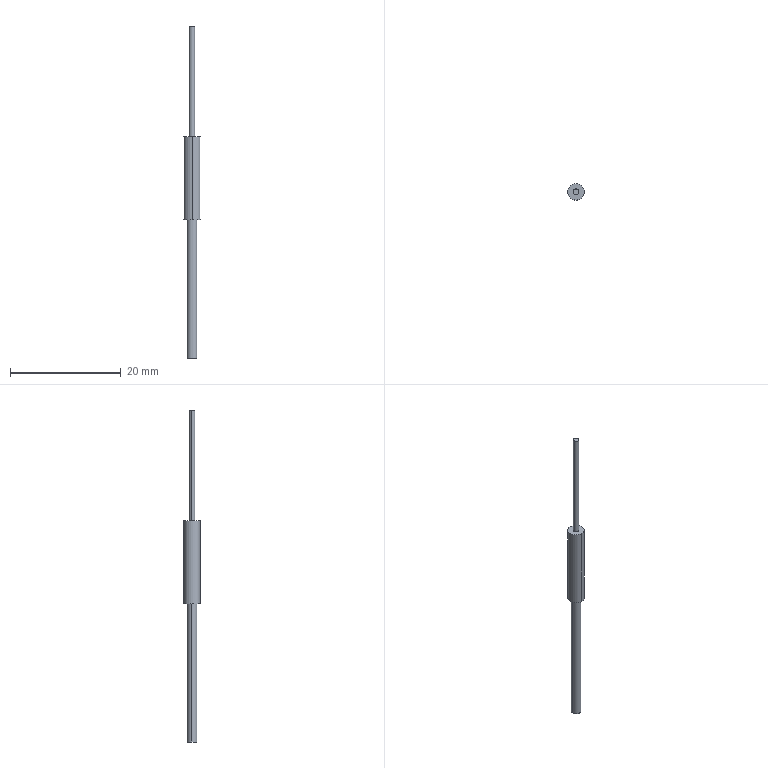Part | SolidWorks | features BaseBody 1 | 1 solid | 10 faces | box 3 x 3 x 60 mm | volume 185.354 mm3 | cylinder 6 | plane 4 | commonest cylinder face diameters 1 x2 1.8 x2 3 x2
STEP:
#1=CARTESIAN_POINT('',(0.03543,0.,-0.9843));
#2=VERTEX_POINT('',#1);
#3=CARTESIAN_POINT('',(-0.03543,0.,-0.9843));
#4=VERTEX_POINT('',#3);
#5=CARTESIAN_POINT('',(0.,0.,-0.9843));
#6=DIRECTION('',(0.,0.,1.));
#7=DIRECTION('',(1.,0.,0.));
#8=AXIS2_PLACEMENT_3D('',#5,#6,#7);
#9=CIRCLE('',#8,0.03543);
#10=EDGE_CURVE('',#2,#4,#9,.T.);
#11=ORIENTED_EDGE('',*,*,#10,.T.);
#12=CARTESIAN_POINT('',(-0.03543,0.,0.));
#13=VERTEX_POINT('',#12);
#14=CARTESIAN_POINT('',(-0.03543,0.,-0.9843));
#15=DIRECTION('',(0.,0.,1.));
#16=VECTOR('',#15,39.37);
#17=LINE('',#14,#16);
#18=EDGE_CURVE('',#4,#13,#17,.T.);
#19=ORIENTED_EDGE('',*,*,#18,.T.);
#20=CARTESIAN_POINT('',(0.03543,0.,0.));
#21=VERTEX_POINT('',#20);
#22=CARTESIAN_POINT('',(0.,0.,0.));
#23=DIRECTION('',(0.,0.,-1.));
#24=DIRECTION('',(1.,0.,0.));
#25=AXIS2_PLACEMENT_3D('',#22,#23,#24);
#26=CIRCLE('',#25,0.03543);
#27=EDGE_CURVE('',#13,#21,#26,.T.);
#28=ORIENTED_EDGE('',*,*,#27,.T.);
#29=CARTESIAN_POINT('',(0.03543,0.,-0.9843));
#30=DIRECTION('',(0.,0.,1.));
#31=VECTOR('',#30,39.37);
#32=LINE('',#29,#31);
#33=EDGE_CURVE('',#2,#21,#32,.T.);
#34=ORIENTED_EDGE('',*,*,#33,.F.);
#35=EDGE_LOOP('',(#11,#19,#28,#34));
#36=FACE_OUTER_BOUND('',#35,.T.);
#37=CARTESIAN_POINT('',(0.,0.,-0.9843));
#38=DIRECTION('',(0.,0.,1.));
#39=DIRECTION('',(1.,0.,0.));
#40=AXIS2_PLACEMENT_3D('',#37,#38,#39);
#41=CYLINDRICAL_SURFACE('',#40,0.03543);
#42=ADVANCED_FACE('',(#36),#41,.T.);
#43=CARTESIAN_POINT('',(0.,0.05906,0.5906));
#44=VERTEX_POINT('',#43);
#45=CARTESIAN_POINT('',(0.,-0.05906,0.5906));
#46=VERTEX_POINT('',#45);
#47=CARTESIAN_POINT('',(0.,0.,0.5906));
#48=DIRECTION('',(0.,0.,-1.));
#49=DIRECTION('',(0.,1.,0.));
#50=AXIS2_PLACEMENT_3D('',#47,#48,#49);
#51=CIRCLE('',#50,0.05906);
#52=EDGE_CURVE('',#44,#46,#51,.T.);
#53=ORIENTED_EDGE('',*,*,#52,.T.);
#54=CARTESIAN_POINT('',(0.,-0.05906,0.));
#55=VERTEX_POINT('',#54);
#56=CARTESIAN_POINT('',(0.,-0.05906,0.5906));
#57=DIRECTION('',(0.,0.,-1.));
#58=VECTOR('',#57,39.37);
#59=LINE('',#56,#58);
#60=EDGE_CURVE('',#46,#55,#59,.T.);
#61=ORIENTED_EDGE('',*,*,#60,.T.);
#62=CARTESIAN_POINT('',(0.,0.05906,0.));
#63=VERTEX_POINT('',#62);
#64=CARTESIAN_POINT('',(0.,0.,0.));
#65=DIRECTION('',(0.,0.,1.));
#66=DIRECTION('',(0.,1.,0.));
#67=AXIS2_PLACEMENT_3D('',#64,#65,#66);
#68=CIRCLE('',#67,0.05906);
#69=EDGE_CURVE('',#55,#63,#68,.T.);
#70=ORIENTED_EDGE('',*,*,#69,.T.);
#71=CARTESIAN_POINT('',(0.,0.05906,0.5906));
#72=DIRECTION('',(0.,0.,-1.));
#73=VECTOR('',#72,39.37);
#74=LINE('',#71,#73);
#75=EDGE_CURVE('',#44,#63,#74,.T.);
#76=ORIENTED_EDGE('',*,*,#75,.F.);
#77=EDGE_LOOP('',(#53,#61,#70,#76));
#78=FACE_OUTER_BOUND('',#77,.T.);
#79=CARTESIAN_POINT('',(0.,0.,0.5906));
#80=DIRECTION('',(0.,0.,-1.));
#81=DIRECTION('',(0.,1.,0.));
#82=AXIS2_PLACEMENT_3D('',#79,#80,#81);
#83=CYLINDRICAL_SURFACE('',#82,0.05906);
#84=ADVANCED_FACE('',(#78),#83,.T.);
#85=CARTESIAN_POINT('',(-0.01969,0.,1.378));
#86=VERTEX_POINT('',#85);
#87=CARTESIAN_POINT('',(0.01969,0.,1.378));
#88=VERTEX_POINT('',#87);
#89=CARTESIAN_POINT('',(0.,0.,1.378));
#90=DIRECTION('',(0.,0.,-1.));
#91=DIRECTION('',(-1.,0.,0.));
#92=AXIS2_PLACEMENT_3D('',#89,#90,#91);
#93=CIRCLE('',#92,0.01969);
#94=EDGE_CURVE('',#86,#88,#93,.T.);
#95=ORIENTED_EDGE('',*,*,#94,.T.);
#96=CARTESIAN_POINT('',(0.01969,0.,0.5906));
#97=VERTEX_POINT('',#96);
#98=CARTESIAN_POINT('',(0.01969,0.,1.378));
#99=DIRECTION('',(0.,0.,-1.));
#100=VECTOR('',#99,39.37);
#101=LINE('',#98,#100);
#102=EDGE_CURVE('',#88,#97,#101,.T.);
#103=ORIENTED_EDGE('',*,*,#102,.T.);
#104=CARTESIAN_POINT('',(-0.01969,0.,0.5906));
#105=VERTEX_POINT('',#104);
#106=CARTESIAN_POINT('',(0.,0.,0.5906));
#107=DIRECTION('',(0.,0.,-1.));
#108=DIRECTION('',(-1.,0.,0.));
#109=AXIS2_PLACEMENT_3D('',#106,#107,#108);
#110=CIRCLE('',#109,0.01969);
#111=EDGE_CURVE('',#105,#97,#110,.T.);
#112=ORIENTED_EDGE('',*,*,#111,.F.);
#113=CARTESIAN_POINT('',(-0.01969,0.,1.378));
#114=DIRECTION('',(0.,0.,-1.));
#115=VECTOR('',#114,39.37);
#116=LINE('',#113,#115);
#117=EDGE_CURVE('',#86,#105,#116,.T.);
#118=ORIENTED_EDGE('',*,*,#117,.F.);
#119=EDGE_LOOP('',(#95,#103,#112,#118));
#120=FACE_OUTER_BOUND('',#119,.T.);
#121=CARTESIAN_POINT('',(0.,0.,1.378));
#122=DIRECTION('',(0.,0.,-1.));
#123=DIRECTION('',(-1.,0.,0.));
#124=AXIS2_PLACEMENT_3D('',#121,#122,#123);
#125=CYLINDRICAL_SURFACE('',#124,0.01969);
#126=ADVANCED_FACE('',(#120),#125,.T.);
#127=ORIENTED_EDGE('',*,*,#18,.F.);
#128=CARTESIAN_POINT('',(0.,0.,-0.9843));
#129=DIRECTION('',(0.,0.,1.));
#130=DIRECTION('',(1.,0.,0.));
#131=AXIS2_PLACEMENT_3D('',#128,#129,#130);
#132=CIRCLE('',#131,0.03543);
#133=EDGE_CURVE('',#4,#2,#132,.T.);
#134=ORIENTED_EDGE('',*,*,#133,.T.);
#135=ORIENTED_EDGE('',*,*,#33,.T.);
#136=CARTESIAN_POINT('',(0.,0.,0.));
#137=DIRECTION('',(0.,0.,-1.));
#138=DIRECTION('',(1.,0.,0.));
#139=AXIS2_PLACEMENT_3D('',#136,#137,#138);
#140=CIRCLE('',#139,0.03543);
#141=EDGE_CURVE('',#21,#13,#140,.T.);
#142=ORIENTED_EDGE('',*,*,#141,.T.);
#143=EDGE_LOOP('',(#127,#134,#135,#142));
#144=FACE_OUTER_BOUND('',#143,.T.);
#145=CARTESIAN_POINT('',(0.,0.,-0.9843));
#146=DIRECTION('',(0.,0.,1.));
#147=DIRECTION('',(1.,0.,0.));
#148=AXIS2_PLACEMENT_3D('',#145,#146,#147);
#149=CYLINDRICAL_SURFACE('',#148,0.03543);
#150=ADVANCED_FACE('',(#144),#149,.T.);
#151=CARTESIAN_POINT('',(0.,0.,0.));
#152=DIRECTION('',(0.,0.,1.));
#153=DIRECTION('',(0.,1.,0.));
#154=AXIS2_PLACEMENT_3D('',#151,#152,#153);
#155=CIRCLE('',#154,0.05906);
#156=EDGE_CURVE('',#63,#55,#155,.T.);
#157=ORIENTED_EDGE('',*,*,#156,.F.);
#158=ORIENTED_EDGE('',*,*,#69,.F.);
#159=EDGE_LOOP('',(#157,#158));
#160=FACE_OUTER_BOUND('',#159,.T.);
#161=ORIENTED_EDGE('',*,*,#141,.F.);
#162=ORIENTED_EDGE('',*,*,#27,.F.);
#163=EDGE_LOOP('',(#161,#162));
#164=FACE_BOUND('',#163,.T.);
#165=CARTESIAN_POINT('',(-0.05976,-0.05976,0.));
#166=DIRECTION('',(0.,0.,1.));
#167=DIRECTION('',(1.,0.,0.));
#168=AXIS2_PLACEMENT_3D('',#165,#166,#167);
#169=PLANE('',#168);
#170=ADVANCED_FACE('',(#160,#164),#169,.F.);
#171=ORIENTED_EDGE('',*,*,#10,.F.);
#172=ORIENTED_EDGE('',*,*,#133,.F.);
#173=EDGE_LOOP('',(#171,#172));
#174=FACE_OUTER_BOUND('',#173,.T.);
#175=CARTESIAN_POINT('',(0.03586,-0.03586,-0.9843));
#176=DIRECTION('',(0.,0.,-1.));
#177=DIRECTION('',(-1.,0.,0.));
#178=AXIS2_PLACEMENT_3D('',#175,#176,#177);
#179=PLANE('',#178);
#180=ADVANCED_FACE('',(#174),#179,.T.);
#181=ORIENTED_EDGE('',*,*,#60,.F.);
#182=CARTESIAN_POINT('',(0.,0.,0.5906));
#183=DIRECTION('',(0.,0.,-1.));
#184=DIRECTION('',(0.,1.,0.));
#185=AXIS2_PLACEMENT_3D('',#182,#183,#184);
#186=CIRCLE('',#185,0.05906);
#187=EDGE_CURVE('',#46,#44,#186,.T.);
#188=ORIENTED_EDGE('',*,*,#187,.T.);
#189=ORIENTED_EDGE('',*,*,#75,.T.);
#190=ORIENTED_EDGE('',*,*,#156,.T.);
#191=EDGE_LOOP('',(#181,#188,#189,#190));
#192=FACE_OUTER_BOUND('',#191,.T.);
#193=CARTESIAN_POINT('',(0.,0.,0.5906));
#194=DIRECTION('',(0.,0.,-1.));
#195=DIRECTION('',(0.,1.,0.));
#196=AXIS2_PLACEMENT_3D('',#193,#194,#195);
#197=CYLINDRICAL_SURFACE('',#196,0.05906);
#198=ADVANCED_FACE('',(#192),#197,.T.);
#199=ORIENTED_EDGE('',*,*,#111,.T.);
#200=CARTESIAN_POINT('',(0.,0.,0.5906));
#201=DIRECTION('',(0.,0.,-1.));
#202=DIRECTION('',(-1.,0.,0.));
#203=AXIS2_PLACEMENT_3D('',#200,#201,#202);
#204=CIRCLE('',#203,0.01969);
#205=EDGE_CURVE('',#97,#105,#204,.T.);
#206=ORIENTED_EDGE('',*,*,#205,.T.);
#207=EDGE_LOOP('',(#199,#206));
#208=FACE_BOUND('',#207,.T.);
#209=ORIENTED_EDGE('',*,*,#52,.F.);
#210=ORIENTED_EDGE('',*,*,#187,.F.);
#211=EDGE_LOOP('',(#209,#210));
#212=FACE_OUTER_BOUND('',#211,.T.);
#213=CARTESIAN_POINT('',(-0.05976,-0.05976,0.5906));
#214=DIRECTION('',(0.,0.,1.));
#215=DIRECTION('',(1.,0.,0.));
#216=AXIS2_PLACEMENT_3D('',#213,#214,#215);
#217=PLANE('',#216);
#218=ADVANCED_FACE('',(#208,#212),#217,.T.);
#219=ORIENTED_EDGE('',*,*,#102,.F.);
#220=CARTESIAN_POINT('',(0.,0.,1.378));
#221=DIRECTION('',(0.,0.,-1.));
#222=DIRECTION('',(-1.,0.,0.));
#223=AXIS2_PLACEMENT_3D('',#220,#221,#222);
#224=CIRCLE('',#223,0.01969);
#225=EDGE_CURVE('',#88,#86,#224,.T.);
#226=ORIENTED_EDGE('',*,*,#225,.T.);
#227=ORIENTED_EDGE('',*,*,#117,.T.);
#228=ORIENTED_EDGE('',*,*,#205,.F.);
#229=EDGE_LOOP('',(#219,#226,#227,#228));
#230=FACE_OUTER_BOUND('',#229,.T.);
#231=CARTESIAN_POINT('',(0.,0.,1.378));
#232=DIRECTION('',(0.,0.,-1.));
#233=DIRECTION('',(-1.,0.,0.));
#234=AXIS2_PLACEMENT_3D('',#231,#232,#233);
#235=CYLINDRICAL_SURFACE('',#234,0.01969);
#236=ADVANCED_FACE('',(#230),#235,.T.);
#237=ORIENTED_EDGE('',*,*,#94,.F.);
#238=ORIENTED_EDGE('',*,*,#225,.F.);
#239=EDGE_LOOP('',(#237,#238));
#240=FACE_OUTER_BOUND('',#239,.T.);
#241=CARTESIAN_POINT('',(0.,0.,1.378));
#242=DIRECTION('',(0.,0.,1.));
#243=DIRECTION('',(1.,0.,0.));
#244=AXIS2_PLACEMENT_3D('',#241,#242,#243);
#245=PLANE('',#244);
#246=ADVANCED_FACE('',(#240),#245,.T.);
#247=CLOSED_SHELL('',(#42,#84,#126,#150,#170,#180,#198,#218,#236,#246));
#248=MANIFOLD_SOLID_BREP('',#247);
#249=CARTESIAN_POINT('',(0.,0.,0.));
#250=DIRECTION('',(0.,0.,1.));
#251=DIRECTION('',(1.,0.,0.));
#252=AXIS2_PLACEMENT_3D('',#249,#250,#251);
#253=(LENGTH_UNIT()NAMED_UNIT(*)SI_UNIT($,.METRE.));
#254=LENGTH_MEASURE_WITH_UNIT(LENGTH_MEASURE(0.0254),#253);
#255=DIMENSIONAL_EXPONENTS(1.,0.,0.,0.,0.,0.,0.);
#256=(CONVERSION_BASED_UNIT('INCH',#254)LENGTH_UNIT()NAMED_UNIT(#255));
#257=UNCERTAINTY_MEASURE_WITH_UNIT(LENGTH_MEASURE(0.00001),#256,'','');
#258=(NAMED_UNIT(*)PLANE_ANGLE_UNIT()SI_UNIT($,.RADIAN.));
#259=(NAMED_UNIT(*)SI_UNIT($,.STERADIAN.)SOLID_ANGLE_UNIT());
#260=(GEOMETRIC_REPRESENTATION_CONTEXT(3)GLOBAL_UNCERTAINTY_ASSIGNED_CONTEXT((#257))GLOBAL_UNIT_ASSIGNED_CONTEXT((#256,#258,#259))REPRESENTATION_CONTEXT('',''));
#261=ADVANCED_BREP_SHAPE_REPRESENTATION('',(#248,#252),#260);